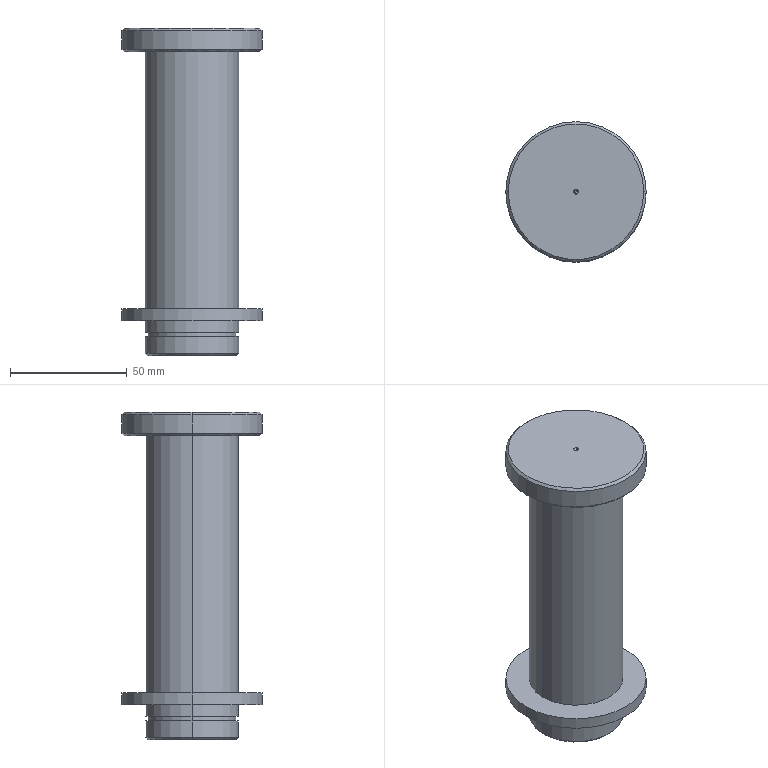Part | SolidWorks | features BaseBody 2 | 2 solids | 29 faces | box 60 x 60 x 140 mm | volume 198937 mm3 | cylinder 12 | cone 10 | plane 7 | commonest cylinder face diameters 40 x6 60 x4 37.5 x2
STEP:
#1=CARTESIAN_POINT('',(29.,0.,60.));
#2=VERTEX_POINT('',#1);
#3=CARTESIAN_POINT('',(-29.,0.,60.));
#4=VERTEX_POINT('',#3);
#5=CARTESIAN_POINT('',(0.,0.,60.));
#6=DIRECTION('',(0.,0.,1.));
#7=DIRECTION('',(1.,0.,0.));
#8=AXIS2_PLACEMENT_3D('',#5,#6,#7);
#9=CIRCLE('',#8,29.);
#10=EDGE_CURVE('',#2,#4,#9,.T.);
#11=ORIENTED_EDGE('',*,*,#10,.T.);
#12=CARTESIAN_POINT('',(-30.,0.,61.));
#13=VERTEX_POINT('',#12);
#14=CARTESIAN_POINT('',(-29.,0.,60.));
#15=DIRECTION('',(-0.7071,0.,0.7071));
#16=VECTOR('',#15,1000.);
#17=LINE('',#14,#16);
#18=EDGE_CURVE('',#4,#13,#17,.T.);
#19=ORIENTED_EDGE('',*,*,#18,.T.);
#20=CARTESIAN_POINT('',(30.,0.,61.));
#21=VERTEX_POINT('',#20);
#22=CARTESIAN_POINT('',(0.,0.,61.));
#23=DIRECTION('',(0.,0.,1.));
#24=DIRECTION('',(1.,0.,0.));
#25=AXIS2_PLACEMENT_3D('',#22,#23,#24);
#26=CIRCLE('',#25,30.);
#27=EDGE_CURVE('',#21,#13,#26,.T.);
#28=ORIENTED_EDGE('',*,*,#27,.F.);
#29=CARTESIAN_POINT('',(29.,0.,60.));
#30=DIRECTION('',(0.7071,0.,0.7071));
#31=VECTOR('',#30,1000.);
#32=LINE('',#29,#31);
#33=EDGE_CURVE('',#2,#21,#32,.T.);
#34=ORIENTED_EDGE('',*,*,#33,.F.);
#35=EDGE_LOOP('',(#11,#19,#28,#34));
#36=FACE_OUTER_BOUND('',#35,.T.);
#37=CARTESIAN_POINT('',(0.,0.,60.));
#38=DIRECTION('',(0.,0.,1.));
#39=DIRECTION('',(1.,0.,0.));
#40=AXIS2_PLACEMENT_3D('',#37,#38,#39);
#41=CONICAL_SURFACE('',#40,29.,0.7854);
#42=ADVANCED_FACE('',(#36),#41,.T.);
#43=ORIENTED_EDGE('',*,*,#27,.T.);
#44=CARTESIAN_POINT('',(-30.,0.,69.));
#45=VERTEX_POINT('',#44);
#46=CARTESIAN_POINT('',(-30.,0.,69.));
#47=DIRECTION('',(0.,0.,1.));
#48=VECTOR('',#47,1000.);
#49=LINE('',#46,#48);
#50=EDGE_CURVE('',#13,#45,#49,.T.);
#51=ORIENTED_EDGE('',*,*,#50,.T.);
#52=CARTESIAN_POINT('',(30.,0.,69.));
#53=VERTEX_POINT('',#52);
#54=CARTESIAN_POINT('',(0.,0.,69.));
#55=DIRECTION('',(0.,0.,1.));
#56=DIRECTION('',(1.,0.,0.));
#57=AXIS2_PLACEMENT_3D('',#54,#55,#56);
#58=CIRCLE('',#57,30.);
#59=EDGE_CURVE('',#53,#45,#58,.T.);
#60=ORIENTED_EDGE('',*,*,#59,.F.);
#61=CARTESIAN_POINT('',(30.,0.,69.));
#62=DIRECTION('',(0.,0.,1.));
#63=VECTOR('',#62,1000.);
#64=LINE('',#61,#63);
#65=EDGE_CURVE('',#21,#53,#64,.T.);
#66=ORIENTED_EDGE('',*,*,#65,.F.);
#67=EDGE_LOOP('',(#43,#51,#60,#66));
#68=FACE_OUTER_BOUND('',#67,.T.);
#69=CARTESIAN_POINT('',(0.,0.,69.));
#70=DIRECTION('',(0.,0.,1.));
#71=DIRECTION('',(1.,0.,0.));
#72=AXIS2_PLACEMENT_3D('',#69,#70,#71);
#73=CYLINDRICAL_SURFACE('',#72,30.);
#74=ADVANCED_FACE('',(#68),#73,.T.);
#75=CARTESIAN_POINT('',(29.,0.,70.));
#76=VERTEX_POINT('',#75);
#77=CARTESIAN_POINT('',(-29.,0.,70.));
#78=VERTEX_POINT('',#77);
#79=CARTESIAN_POINT('',(0.,0.,70.));
#80=DIRECTION('',(0.,0.,1.));
#81=DIRECTION('',(1.,0.,0.));
#82=AXIS2_PLACEMENT_3D('',#79,#80,#81);
#83=CIRCLE('',#82,29.);
#84=EDGE_CURVE('',#76,#78,#83,.T.);
#85=ORIENTED_EDGE('',*,*,#84,.F.);
#86=CARTESIAN_POINT('',(30.,0.,69.));
#87=DIRECTION('',(0.7071,0.,-0.7071));
#88=VECTOR('',#87,1000.);
#89=LINE('',#86,#88);
#90=EDGE_CURVE('',#76,#53,#89,.T.);
#91=ORIENTED_EDGE('',*,*,#90,.T.);
#92=ORIENTED_EDGE('',*,*,#59,.T.);
#93=CARTESIAN_POINT('',(-30.,0.,69.));
#94=DIRECTION('',(-0.7071,0.,-0.7071));
#95=VECTOR('',#94,1000.);
#96=LINE('',#93,#95);
#97=EDGE_CURVE('',#78,#45,#96,.T.);
#98=ORIENTED_EDGE('',*,*,#97,.F.);
#99=EDGE_LOOP('',(#85,#91,#92,#98));
#100=FACE_OUTER_BOUND('',#99,.T.);
#101=CARTESIAN_POINT('',(0.,0.,69.));
#102=DIRECTION('',(0.,0.,-1.));
#103=DIRECTION('',(-1.,0.,0.));
#104=AXIS2_PLACEMENT_3D('',#101,#102,#103);
#105=CONICAL_SURFACE('',#104,30.,0.7854);
#106=ADVANCED_FACE('',(#100),#105,.T.);
#107=CARTESIAN_POINT('',(0.,0.,69.));
#108=VERTEX_POINT('',#107);
#109=CARTESIAN_POINT('',(1.,0.,70.));
#110=VERTEX_POINT('',#109);
#111=CARTESIAN_POINT('',(1.,0.,70.));
#112=DIRECTION('',(0.7071,0.,0.7071));
#113=VECTOR('',#112,1000.);
#114=LINE('',#111,#113);
#115=EDGE_CURVE('',#108,#110,#114,.T.);
#116=ORIENTED_EDGE('',*,*,#115,.F.);
#117=CARTESIAN_POINT('',(-1.,0.,70.));
#118=VERTEX_POINT('',#117);
#119=CARTESIAN_POINT('',(-1.,0.,70.));
#120=DIRECTION('',(-0.7071,0.,0.7071));
#121=VECTOR('',#120,1000.);
#122=LINE('',#119,#121);
#123=EDGE_CURVE('',#108,#118,#122,.T.);
#124=ORIENTED_EDGE('',*,*,#123,.T.);
#125=CARTESIAN_POINT('',(0.,0.,70.));
#126=DIRECTION('',(0.,0.,1.));
#127=DIRECTION('',(1.,0.,0.));
#128=AXIS2_PLACEMENT_3D('',#125,#126,#127);
#129=CIRCLE('',#128,1.);
#130=EDGE_CURVE('',#118,#110,#129,.T.);
#131=ORIENTED_EDGE('',*,*,#130,.T.);
#132=EDGE_LOOP('',(#116,#124,#131));
#133=FACE_OUTER_BOUND('',#132,.T.);
#134=CARTESIAN_POINT('',(0.,0.,70.));
#135=DIRECTION('',(0.,0.,1.));
#136=DIRECTION('',(1.,0.,0.));
#137=AXIS2_PLACEMENT_3D('',#134,#135,#136);
#138=CONICAL_SURFACE('',#137,1.,0.7854);
#139=ADVANCED_FACE('',(#133),#138,.F.);
#140=CARTESIAN_POINT('',(0.,0.,-69.));
#141=VERTEX_POINT('',#140);
#142=CARTESIAN_POINT('',(-1.,0.,-70.));
#143=VERTEX_POINT('',#142);
#144=CARTESIAN_POINT('',(0.,0.,-69.));
#145=DIRECTION('',(-0.7071,0.,-0.7071));
#146=VECTOR('',#145,1000.);
#147=LINE('',#144,#146);
#148=EDGE_CURVE('',#141,#143,#147,.T.);
#149=ORIENTED_EDGE('',*,*,#148,.F.);
#150=CARTESIAN_POINT('',(1.,0.,-70.));
#151=VERTEX_POINT('',#150);
#152=CARTESIAN_POINT('',(0.,0.,-69.));
#153=DIRECTION('',(0.7071,0.,-0.7071));
#154=VECTOR('',#153,1000.);
#155=LINE('',#152,#154);
#156=EDGE_CURVE('',#141,#151,#155,.T.);
#157=ORIENTED_EDGE('',*,*,#156,.T.);
#158=CARTESIAN_POINT('',(0.,0.,-70.));
#159=DIRECTION('',(0.,0.,1.));
#160=DIRECTION('',(1.,0.,0.));
#161=AXIS2_PLACEMENT_3D('',#158,#159,#160);
#162=CIRCLE('',#161,1.);
#163=EDGE_CURVE('',#143,#151,#162,.T.);
#164=ORIENTED_EDGE('',*,*,#163,.F.);
#165=EDGE_LOOP('',(#149,#157,#164));
#166=FACE_OUTER_BOUND('',#165,.T.);
#167=CARTESIAN_POINT('',(0.,0.,-1069.));
#168=DIRECTION('',(0.,0.,-1.));
#169=DIRECTION('',(-1.,0.,0.));
#170=AXIS2_PLACEMENT_3D('',#167,#168,#169);
#171=CONICAL_SURFACE('',#170,1000.,0.7854);
#172=ADVANCED_FACE('',(#166),#171,.F.);
#173=CARTESIAN_POINT('',(19.,0.,-70.));
#174=VERTEX_POINT('',#173);
#175=CARTESIAN_POINT('',(-19.,0.,-70.));
#176=VERTEX_POINT('',#175);
#177=CARTESIAN_POINT('',(0.,0.,-70.));
#178=DIRECTION('',(0.,0.,1.));
#179=DIRECTION('',(1.,0.,0.));
#180=AXIS2_PLACEMENT_3D('',#177,#178,#179);
#181=CIRCLE('',#180,19.);
#182=EDGE_CURVE('',#174,#176,#181,.T.);
#183=ORIENTED_EDGE('',*,*,#182,.T.);
#184=CARTESIAN_POINT('',(-20.,0.,-69.));
#185=VERTEX_POINT('',#184);
#186=CARTESIAN_POINT('',(-19.,0.,-70.));
#187=DIRECTION('',(-0.7071,0.,0.7071));
#188=VECTOR('',#187,1000.);
#189=LINE('',#186,#188);
#190=EDGE_CURVE('',#176,#185,#189,.T.);
#191=ORIENTED_EDGE('',*,*,#190,.T.);
#192=CARTESIAN_POINT('',(20.,0.,-69.));
#193=VERTEX_POINT('',#192);
#194=CARTESIAN_POINT('',(0.,0.,-69.));
#195=DIRECTION('',(0.,0.,1.));
#196=DIRECTION('',(1.,0.,0.));
#197=AXIS2_PLACEMENT_3D('',#194,#195,#196);
#198=CIRCLE('',#197,20.);
#199=EDGE_CURVE('',#193,#185,#198,.T.);
#200=ORIENTED_EDGE('',*,*,#199,.F.);
#201=CARTESIAN_POINT('',(19.,0.,-70.));
#202=DIRECTION('',(0.7071,0.,0.7071));
#203=VECTOR('',#202,1000.);
#204=LINE('',#201,#203);
#205=EDGE_CURVE('',#174,#193,#204,.T.);
#206=ORIENTED_EDGE('',*,*,#205,.F.);
#207=EDGE_LOOP('',(#183,#191,#200,#206));
#208=FACE_OUTER_BOUND('',#207,.T.);
#209=CARTESIAN_POINT('',(0.,0.,-70.));
#210=DIRECTION('',(0.,0.,1.));
#211=DIRECTION('',(1.,0.,0.));
#212=AXIS2_PLACEMENT_3D('',#209,#210,#211);
#213=CONICAL_SURFACE('',#212,19.,0.7854);
#214=ADVANCED_FACE('',(#208),#213,.T.);
#215=ORIENTED_EDGE('',*,*,#199,.T.);
#216=CARTESIAN_POINT('',(-20.,0.,-62.));
#217=VERTEX_POINT('',#216);
#218=CARTESIAN_POINT('',(-20.,0.,69.));
#219=DIRECTION('',(0.,0.,1.));
#220=VECTOR('',#219,1000.);
#221=LINE('',#218,#220);
#222=EDGE_CURVE('',#185,#217,#221,.T.);
#223=ORIENTED_EDGE('',*,*,#222,.T.);
#224=CARTESIAN_POINT('',(20.,0.,-62.));
#225=VERTEX_POINT('',#224);
#226=CARTESIAN_POINT('',(0.,0.,-62.));
#227=DIRECTION('',(0.,0.,1.));
#228=DIRECTION('',(1.,0.,0.));
#229=AXIS2_PLACEMENT_3D('',#226,#227,#228);
#230=CIRCLE('',#229,20.);
#231=EDGE_CURVE('',#225,#217,#230,.T.);
#232=ORIENTED_EDGE('',*,*,#231,.F.);
#233=CARTESIAN_POINT('',(20.,0.,69.));
#234=DIRECTION('',(0.,0.,1.));
#235=VECTOR('',#234,1000.);
#236=LINE('',#233,#235);
#237=EDGE_CURVE('',#193,#225,#236,.T.);
#238=ORIENTED_EDGE('',*,*,#237,.F.);
#239=EDGE_LOOP('',(#215,#223,#232,#238));
#240=FACE_OUTER_BOUND('',#239,.T.);
#241=CARTESIAN_POINT('',(0.,0.,69.));
#242=DIRECTION('',(0.,0.,1.));
#243=DIRECTION('',(1.,0.,0.));
#244=AXIS2_PLACEMENT_3D('',#241,#242,#243);
#245=CYLINDRICAL_SURFACE('',#244,20.);
#246=ADVANCED_FACE('',(#240),#245,.T.);
#247=CARTESIAN_POINT('',(18.75,0.,-62.));
#248=VERTEX_POINT('',#247);
#249=CARTESIAN_POINT('',(-18.75,0.,-62.));
#250=VERTEX_POINT('',#249);
#251=CARTESIAN_POINT('',(0.,0.,-62.));
#252=DIRECTION('',(0.,0.,1.));
#253=DIRECTION('',(1.,0.,0.));
#254=AXIS2_PLACEMENT_3D('',#251,#252,#253);
#255=CIRCLE('',#254,18.75);
#256=EDGE_CURVE('',#248,#250,#255,.T.);
#257=ORIENTED_EDGE('',*,*,#256,.T.);
#258=CARTESIAN_POINT('',(-18.75,0.,-60.));
#259=VERTEX_POINT('',#258);
#260=CARTESIAN_POINT('',(-18.75,0.,69.));
#261=DIRECTION('',(0.,0.,1.));
#262=VECTOR('',#261,1000.);
#263=LINE('',#260,#262);
#264=EDGE_CURVE('',#250,#259,#263,.T.);
#265=ORIENTED_EDGE('',*,*,#264,.T.);
#266=CARTESIAN_POINT('',(18.75,0.,-60.));
#267=VERTEX_POINT('',#266);
#268=CARTESIAN_POINT('',(0.,0.,-60.));
#269=DIRECTION('',(0.,0.,1.));
#270=DIRECTION('',(1.,0.,0.));
#271=AXIS2_PLACEMENT_3D('',#268,#269,#270);
#272=CIRCLE('',#271,18.75);
#273=EDGE_CURVE('',#267,#259,#272,.T.);
#274=ORIENTED_EDGE('',*,*,#273,.F.);
#275=CARTESIAN_POINT('',(18.75,0.,69.));
#276=DIRECTION('',(0.,0.,1.));
#277=VECTOR('',#276,1000.);
#278=LINE('',#275,#277);
#279=EDGE_CURVE('',#248,#267,#278,.T.);
#280=ORIENTED_EDGE('',*,*,#279,.F.);
#281=EDGE_LOOP('',(#257,#265,#274,#280));
#282=FACE_OUTER_BOUND('',#281,.T.);
#283=CARTESIAN_POINT('',(0.,0.,69.));
#284=DIRECTION('',(0.,0.,1.));
#285=DIRECTION('',(1.,0.,0.));
#286=AXIS2_PLACEMENT_3D('',#283,#284,#285);
#287=CYLINDRICAL_SURFACE('',#286,18.75);
#288=ADVANCED_FACE('',(#282),#287,.T.);
#289=CARTESIAN_POINT('',(20.,0.,-60.));
#290=VERTEX_POINT('',#289);
#291=CARTESIAN_POINT('',(-20.,0.,-60.));
#292=VERTEX_POINT('',#291);
#293=CARTESIAN_POINT('',(0.,0.,-60.));
#294=DIRECTION('',(0.,0.,1.));
#295=DIRECTION('',(1.,0.,0.));
#296=AXIS2_PLACEMENT_3D('',#293,#294,#295);
#297=CIRCLE('',#296,20.);
#298=EDGE_CURVE('',#290,#292,#297,.T.);
#299=ORIENTED_EDGE('',*,*,#298,.T.);
#300=CARTESIAN_POINT('',(-20.,0.,60.));
#301=VERTEX_POINT('',#300);
#302=CARTESIAN_POINT('',(-20.,0.,69.));
#303=DIRECTION('',(0.,0.,1.));
#304=VECTOR('',#303,1000.);
#305=LINE('',#302,#304);
#306=EDGE_CURVE('',#292,#301,#305,.T.);
#307=ORIENTED_EDGE('',*,*,#306,.T.);
#308=CARTESIAN_POINT('',(20.,0.,60.));
#309=VERTEX_POINT('',#308);
#310=CARTESIAN_POINT('',(0.,0.,60.));
#311=DIRECTION('',(0.,0.,1.));
#312=DIRECTION('',(1.,0.,0.));
#313=AXIS2_PLACEMENT_3D('',#310,#311,#312);
#314=CIRCLE('',#313,20.);
#315=EDGE_CURVE('',#309,#301,#314,.T.);
#316=ORIENTED_EDGE('',*,*,#315,.F.);
#317=CARTESIAN_POINT('',(20.,0.,69.));
#318=DIRECTION('',(0.,0.,1.));
#319=VECTOR('',#318,1000.);
#320=LINE('',#317,#319);
#321=EDGE_CURVE('',#290,#309,#320,.T.);
#322=ORIENTED_EDGE('',*,*,#321,.F.);
#323=EDGE_LOOP('',(#299,#307,#316,#322));
#324=FACE_OUTER_BOUND('',#323,.T.);
#325=CARTESIAN_POINT('',(0.,0.,69.));
#326=DIRECTION('',(0.,0.,1.));
#327=DIRECTION('',(1.,0.,0.));
#328=AXIS2_PLACEMENT_3D('',#325,#326,#327);
#329=CYLINDRICAL_SURFACE('',#328,20.);
#330=ADVANCED_FACE('',(#324),#329,.T.);
#331=ORIENTED_EDGE('',*,*,#306,.F.);
#332=CARTESIAN_POINT('',(0.,0.,-60.));
#333=DIRECTION('',(0.,0.,1.));
#334=DIRECTION('',(1.,0.,0.));
#335=AXIS2_PLACEMENT_3D('',#332,#333,#334);
#336=CIRCLE('',#335,20.);
#337=EDGE_CURVE('',#292,#290,#336,.T.);
#338=ORIENTED_EDGE('',*,*,#337,.T.);
#339=ORIENTED_EDGE('',*,*,#321,.T.);
#340=CARTESIAN_POINT('',(0.,0.,60.));
#341=DIRECTION('',(0.,0.,1.));
#342=DIRECTION('',(1.,0.,0.));
#343=AXIS2_PLACEMENT_3D('',#340,#341,#342);
#344=CIRCLE('',#343,20.);
#345=EDGE_CURVE('',#301,#309,#344,.T.);
#346=ORIENTED_EDGE('',*,*,#345,.F.);
#347=EDGE_LOOP('',(#331,#338,#339,#346));
#348=FACE_OUTER_BOUND('',#347,.T.);
#349=CARTESIAN_POINT('',(0.,0.,69.));
#350=DIRECTION('',(0.,0.,1.));
#351=DIRECTION('',(1.,0.,0.));
#352=AXIS2_PLACEMENT_3D('',#349,#350,#351);
#353=CYLINDRICAL_SURFACE('',#352,20.);
#354=ADVANCED_FACE('',(#348),#353,.T.);
#355=ORIENTED_EDGE('',*,*,#298,.F.);
#356=ORIENTED_EDGE('',*,*,#337,.F.);
#357=EDGE_LOOP('',(#355,#356));
#358=FACE_OUTER_BOUND('',#357,.T.);
#359=ORIENTED_EDGE('',*,*,#273,.T.);
#360=CARTESIAN_POINT('',(0.,0.,-60.));
#361=DIRECTION('',(0.,0.,1.));
#362=DIRECTION('',(1.,0.,0.));
#363=AXIS2_PLACEMENT_3D('',#360,#361,#362);
#364=CIRCLE('',#363,18.75);
#365=EDGE_CURVE('',#259,#267,#364,.T.);
#366=ORIENTED_EDGE('',*,*,#365,.T.);
#367=EDGE_LOOP('',(#359,#366));
#368=FACE_BOUND('',#367,.T.);
#369=CARTESIAN_POINT('',(0.,20.,-60.));
#370=DIRECTION('',(0.,0.,1.));
#371=DIRECTION('',(1.,0.,0.));
#372=AXIS2_PLACEMENT_3D('',#369,#370,#371);
#373=PLANE('',#372);
#374=ADVANCED_FACE('',(#358,#368),#373,.F.);
#375=ORIENTED_EDGE('',*,*,#264,.F.);
#376=CARTESIAN_POINT('',(0.,0.,-62.));
#377=DIRECTION('',(0.,0.,1.));
#378=DIRECTION('',(1.,0.,0.));
#379=AXIS2_PLACEMENT_3D('',#376,#377,#378);
#380=CIRCLE('',#379,18.75);
#381=EDGE_CURVE('',#250,#248,#380,.T.);
#382=ORIENTED_EDGE('',*,*,#381,.T.);
#383=ORIENTED_EDGE('',*,*,#279,.T.);
#384=ORIENTED_EDGE('',*,*,#365,.F.);
#385=EDGE_LOOP('',(#375,#382,#383,#384));
#386=FACE_OUTER_BOUND('',#385,.T.);
#387=CARTESIAN_POINT('',(0.,0.,69.));
#388=DIRECTION('',(0.,0.,1.));
#389=DIRECTION('',(1.,0.,0.));
#390=AXIS2_PLACEMENT_3D('',#387,#388,#389);
#391=CYLINDRICAL_SURFACE('',#390,18.75);
#392=ADVANCED_FACE('',(#386),#391,.T.);
#393=ORIENTED_EDGE('',*,*,#256,.F.);
#394=ORIENTED_EDGE('',*,*,#381,.F.);
#395=EDGE_LOOP('',(#393,#394));
#396=FACE_BOUND('',#395,.T.);
#397=ORIENTED_EDGE('',*,*,#231,.T.);
#398=CARTESIAN_POINT('',(0.,0.,-62.));
#399=DIRECTION('',(0.,0.,1.));
#400=DIRECTION('',(1.,0.,0.));
#401=AXIS2_PLACEMENT_3D('',#398,#399,#400);
#402=CIRCLE('',#401,20.);
#403=EDGE_CURVE('',#217,#225,#402,.T.);
#404=ORIENTED_EDGE('',*,*,#403,.T.);
#405=EDGE_LOOP('',(#397,#404));
#406=FACE_OUTER_BOUND('',#405,.T.);
#407=CARTESIAN_POINT('',(0.,18.75,-62.));
#408=DIRECTION('',(0.,0.,-1.));
#409=DIRECTION('',(-1.,0.,0.));
#410=AXIS2_PLACEMENT_3D('',#407,#408,#409);
#411=PLANE('',#410);
#412=ADVANCED_FACE('',(#396,#406),#411,.F.);
#413=ORIENTED_EDGE('',*,*,#222,.F.);
#414=CARTESIAN_POINT('',(0.,0.,-69.));
#415=DIRECTION('',(0.,0.,1.));
#416=DIRECTION('',(1.,0.,0.));
#417=AXIS2_PLACEMENT_3D('',#414,#415,#416);
#418=CIRCLE('',#417,20.);
#419=EDGE_CURVE('',#185,#193,#418,.T.);
#420=ORIENTED_EDGE('',*,*,#419,.T.);
#421=ORIENTED_EDGE('',*,*,#237,.T.);
#422=ORIENTED_EDGE('',*,*,#403,.F.);
#423=EDGE_LOOP('',(#413,#420,#421,#422));
#424=FACE_OUTER_BOUND('',#423,.T.);
#425=CARTESIAN_POINT('',(0.,0.,69.));
#426=DIRECTION('',(0.,0.,1.));
#427=DIRECTION('',(1.,0.,0.));
#428=AXIS2_PLACEMENT_3D('',#425,#426,#427);
#429=CYLINDRICAL_SURFACE('',#428,20.);
#430=ADVANCED_FACE('',(#424),#429,.T.);
#431=ORIENTED_EDGE('',*,*,#190,.F.);
#432=CARTESIAN_POINT('',(0.,0.,-70.));
#433=DIRECTION('',(0.,0.,1.));
#434=DIRECTION('',(1.,0.,0.));
#435=AXIS2_PLACEMENT_3D('',#432,#433,#434);
#436=CIRCLE('',#435,19.);
#437=EDGE_CURVE('',#176,#174,#436,.T.);
#438=ORIENTED_EDGE('',*,*,#437,.T.);
#439=ORIENTED_EDGE('',*,*,#205,.T.);
#440=ORIENTED_EDGE('',*,*,#419,.F.);
#441=EDGE_LOOP('',(#431,#438,#439,#440));
#442=FACE_OUTER_BOUND('',#441,.T.);
#443=CARTESIAN_POINT('',(0.,0.,-70.));
#444=DIRECTION('',(0.,0.,1.));
#445=DIRECTION('',(1.,0.,0.));
#446=AXIS2_PLACEMENT_3D('',#443,#444,#445);
#447=CONICAL_SURFACE('',#446,19.,0.7854);
#448=ADVANCED_FACE('',(#442),#447,.T.);
#449=ORIENTED_EDGE('',*,*,#182,.F.);
#450=ORIENTED_EDGE('',*,*,#437,.F.);
#451=EDGE_LOOP('',(#449,#450));
#452=FACE_OUTER_BOUND('',#451,.T.);
#453=ORIENTED_EDGE('',*,*,#163,.T.);
#454=CARTESIAN_POINT('',(0.,0.,-70.));
#455=DIRECTION('',(0.,0.,1.));
#456=DIRECTION('',(1.,0.,0.));
#457=AXIS2_PLACEMENT_3D('',#454,#455,#456);
#458=CIRCLE('',#457,1.);
#459=EDGE_CURVE('',#151,#143,#458,.T.);
#460=ORIENTED_EDGE('',*,*,#459,.T.);
#461=EDGE_LOOP('',(#453,#460));
#462=FACE_BOUND('',#461,.T.);
#463=CARTESIAN_POINT('',(0.,19.,-70.));
#464=DIRECTION('',(0.,0.,1.));
#465=DIRECTION('',(1.,0.,0.));
#466=AXIS2_PLACEMENT_3D('',#463,#464,#465);
#467=PLANE('',#466);
#468=ADVANCED_FACE('',(#452,#462),#467,.F.);
#469=ORIENTED_EDGE('',*,*,#156,.F.);
#470=ORIENTED_EDGE('',*,*,#148,.T.);
#471=ORIENTED_EDGE('',*,*,#459,.F.);
#472=EDGE_LOOP('',(#469,#470,#471));
#473=FACE_OUTER_BOUND('',#472,.T.);
#474=CARTESIAN_POINT('',(0.,0.,-1069.));
#475=DIRECTION('',(0.,0.,-1.));
#476=DIRECTION('',(-1.,0.,0.));
#477=AXIS2_PLACEMENT_3D('',#474,#475,#476);
#478=CONICAL_SURFACE('',#477,1000.,0.7854);
#479=ADVANCED_FACE('',(#473),#478,.F.);
#480=ORIENTED_EDGE('',*,*,#123,.F.);
#481=ORIENTED_EDGE('',*,*,#115,.T.);
#482=CARTESIAN_POINT('',(0.,0.,70.));
#483=DIRECTION('',(0.,0.,1.));
#484=DIRECTION('',(1.,0.,0.));
#485=AXIS2_PLACEMENT_3D('',#482,#483,#484);
#486=CIRCLE('',#485,1.);
#487=EDGE_CURVE('',#110,#118,#486,.T.);
#488=ORIENTED_EDGE('',*,*,#487,.T.);
#489=EDGE_LOOP('',(#480,#481,#488));
#490=FACE_OUTER_BOUND('',#489,.T.);
#491=CARTESIAN_POINT('',(0.,0.,70.));
#492=DIRECTION('',(0.,0.,1.));
#493=DIRECTION('',(1.,0.,0.));
#494=AXIS2_PLACEMENT_3D('',#491,#492,#493);
#495=CONICAL_SURFACE('',#494,1.,0.7854);
#496=ADVANCED_FACE('',(#490),#495,.F.);
#497=ORIENTED_EDGE('',*,*,#487,.F.);
#498=ORIENTED_EDGE('',*,*,#130,.F.);
#499=EDGE_LOOP('',(#497,#498));
#500=FACE_BOUND('',#499,.T.);
#501=CARTESIAN_POINT('',(0.,0.,70.));
#502=DIRECTION('',(0.,0.,1.));
#503=DIRECTION('',(1.,0.,0.));
#504=AXIS2_PLACEMENT_3D('',#501,#502,#503);
#505=CIRCLE('',#504,29.);
#506=EDGE_CURVE('',#78,#76,#505,.T.);
#507=ORIENTED_EDGE('',*,*,#506,.T.);
#508=ORIENTED_EDGE('',*,*,#84,.T.);
#509=EDGE_LOOP('',(#507,#508));
#510=FACE_OUTER_BOUND('',#509,.T.);
#511=CARTESIAN_POINT('',(0.,1.,70.));
#512=DIRECTION('',(0.,0.,-1.));
#513=DIRECTION('',(-1.,0.,0.));
#514=AXIS2_PLACEMENT_3D('',#511,#512,#513);
#515=PLANE('',#514);
#516=ADVANCED_FACE('',(#500,#510),#515,.F.);
#517=ORIENTED_EDGE('',*,*,#90,.F.);
#518=ORIENTED_EDGE('',*,*,#506,.F.);
#519=ORIENTED_EDGE('',*,*,#97,.T.);
#520=CARTESIAN_POINT('',(0.,0.,69.));
#521=DIRECTION('',(0.,0.,1.));
#522=DIRECTION('',(1.,0.,0.));
#523=AXIS2_PLACEMENT_3D('',#520,#521,#522);
#524=CIRCLE('',#523,30.);
#525=EDGE_CURVE('',#45,#53,#524,.T.);
#526=ORIENTED_EDGE('',*,*,#525,.T.);
#527=EDGE_LOOP('',(#517,#518,#519,#526));
#528=FACE_OUTER_BOUND('',#527,.T.);
#529=CARTESIAN_POINT('',(0.,0.,69.));
#530=DIRECTION('',(0.,0.,-1.));
#531=DIRECTION('',(-1.,0.,0.));
#532=AXIS2_PLACEMENT_3D('',#529,#530,#531);
#533=CONICAL_SURFACE('',#532,30.,0.7854);
#534=ADVANCED_FACE('',(#528),#533,.T.);
#535=ORIENTED_EDGE('',*,*,#50,.F.);
#536=CARTESIAN_POINT('',(0.,0.,61.));
#537=DIRECTION('',(0.,0.,1.));
#538=DIRECTION('',(1.,0.,0.));
#539=AXIS2_PLACEMENT_3D('',#536,#537,#538);
#540=CIRCLE('',#539,30.);
#541=EDGE_CURVE('',#13,#21,#540,.T.);
#542=ORIENTED_EDGE('',*,*,#541,.T.);
#543=ORIENTED_EDGE('',*,*,#65,.T.);
#544=ORIENTED_EDGE('',*,*,#525,.F.);
#545=EDGE_LOOP('',(#535,#542,#543,#544));
#546=FACE_OUTER_BOUND('',#545,.T.);
#547=CARTESIAN_POINT('',(0.,0.,69.));
#548=DIRECTION('',(0.,0.,1.));
#549=DIRECTION('',(1.,0.,0.));
#550=AXIS2_PLACEMENT_3D('',#547,#548,#549);
#551=CYLINDRICAL_SURFACE('',#550,30.);
#552=ADVANCED_FACE('',(#546),#551,.T.);
#553=ORIENTED_EDGE('',*,*,#18,.F.);
#554=CARTESIAN_POINT('',(0.,0.,60.));
#555=DIRECTION('',(0.,0.,1.));
#556=DIRECTION('',(1.,0.,0.));
#557=AXIS2_PLACEMENT_3D('',#554,#555,#556);
#558=CIRCLE('',#557,29.);
#559=EDGE_CURVE('',#4,#2,#558,.T.);
#560=ORIENTED_EDGE('',*,*,#559,.T.);
#561=ORIENTED_EDGE('',*,*,#33,.T.);
#562=ORIENTED_EDGE('',*,*,#541,.F.);
#563=EDGE_LOOP('',(#553,#560,#561,#562));
#564=FACE_OUTER_BOUND('',#563,.T.);
#565=CARTESIAN_POINT('',(0.,0.,60.));
#566=DIRECTION('',(0.,0.,1.));
#567=DIRECTION('',(1.,0.,0.));
#568=AXIS2_PLACEMENT_3D('',#565,#566,#567);
#569=CONICAL_SURFACE('',#568,29.,0.7854);
#570=ADVANCED_FACE('',(#564),#569,.T.);
#571=ORIENTED_EDGE('',*,*,#10,.F.);
#572=ORIENTED_EDGE('',*,*,#559,.F.);
#573=EDGE_LOOP('',(#571,#572));
#574=FACE_OUTER_BOUND('',#573,.T.);
#575=ORIENTED_EDGE('',*,*,#315,.T.);
#576=ORIENTED_EDGE('',*,*,#345,.T.);
#577=EDGE_LOOP('',(#575,#576));
#578=FACE_BOUND('',#577,.T.);
#579=CARTESIAN_POINT('',(0.,29.,60.));
#580=DIRECTION('',(0.,0.,1.));
#581=DIRECTION('',(1.,0.,0.));
#582=AXIS2_PLACEMENT_3D('',#579,#580,#581);
#583=PLANE('',#582);
#584=ADVANCED_FACE('',(#574,#578),#583,.F.);
#585=CLOSED_SHELL('',(#42,#74,#106,#139,#172,#214,#246,#288,#330,#354,#374,#392,#412,#430,#448,#468,#479,#496,#516,#534,#552,#570,#584));
#586=MANIFOLD_SOLID_BREP('',#585);
#587=CARTESIAN_POINT('',(20.,0.,-50.));
#588=VERTEX_POINT('',#587);
#589=CARTESIAN_POINT('',(-20.,0.,-50.));
#590=VERTEX_POINT('',#589);
#591=CARTESIAN_POINT('',(0.,0.,-50.));
#592=DIRECTION('',(0.,0.,-1.));
#593=DIRECTION('',(-1.,0.,0.));
#594=AXIS2_PLACEMENT_3D('',#591,#592,#593);
#595=CIRCLE('',#594,20.);
#596=EDGE_CURVE('',#588,#590,#595,.T.);
#597=ORIENTED_EDGE('',*,*,#596,.F.);
#598=CARTESIAN_POINT('',(20.,0.,-55.));
#599=VERTEX_POINT('',#598);
#600=CARTESIAN_POINT('',(20.,0.,-50.));
#601=DIRECTION('',(0.,0.,-1.));
#602=VECTOR('',#601,1000.);
#603=LINE('',#600,#602);
#604=EDGE_CURVE('',#588,#599,#603,.T.);
#605=ORIENTED_EDGE('',*,*,#604,.T.);
#606=CARTESIAN_POINT('',(-20.,0.,-55.));
#607=VERTEX_POINT('',#606);
#608=CARTESIAN_POINT('',(0.,0.,-55.));
#609=DIRECTION('',(0.,0.,-1.));
#610=DIRECTION('',(-1.,0.,0.));
#611=AXIS2_PLACEMENT_3D('',#608,#609,#610);
#612=CIRCLE('',#611,20.);
#613=EDGE_CURVE('',#599,#607,#612,.T.);
#614=ORIENTED_EDGE('',*,*,#613,.T.);
#615=CARTESIAN_POINT('',(-20.,0.,-50.));
#616=DIRECTION('',(0.,0.,-1.));
#617=VECTOR('',#616,1000.);
#618=LINE('',#615,#617);
#619=EDGE_CURVE('',#590,#607,#618,.T.);
#620=ORIENTED_EDGE('',*,*,#619,.F.);
#621=EDGE_LOOP('',(#597,#605,#614,#620));
#622=FACE_OUTER_BOUND('',#621,.T.);
#623=CARTESIAN_POINT('',(0.,0.,-50.));
#624=DIRECTION('',(0.,0.,-1.));
#625=DIRECTION('',(-1.,0.,0.));
#626=AXIS2_PLACEMENT_3D('',#623,#624,#625);
#627=CYLINDRICAL_SURFACE('',#626,20.);
#628=ADVANCED_FACE('',(#622),#627,.F.);
#629=CARTESIAN_POINT('',(-30.,0.,-50.));
#630=VERTEX_POINT('',#629);
#631=CARTESIAN_POINT('',(30.,0.,-50.));
#632=VERTEX_POINT('',#631);
#633=CARTESIAN_POINT('',(0.,0.,-50.));
#634=DIRECTION('',(0.,0.,-1.));
#635=DIRECTION('',(-1.,0.,0.));
#636=AXIS2_PLACEMENT_3D('',#633,#634,#635);
#637=CIRCLE('',#636,30.);
#638=EDGE_CURVE('',#630,#632,#637,.T.);
#639=ORIENTED_EDGE('',*,*,#638,.T.);
#640=CARTESIAN_POINT('',(30.,0.,-55.));
#641=VERTEX_POINT('',#640);
#642=CARTESIAN_POINT('',(30.,0.,-50.));
#643=DIRECTION('',(0.,0.,-1.));
#644=VECTOR('',#643,1000.);
#645=LINE('',#642,#644);
#646=EDGE_CURVE('',#632,#641,#645,.T.);
#647=ORIENTED_EDGE('',*,*,#646,.T.);
#648=CARTESIAN_POINT('',(-30.,0.,-55.));
#649=VERTEX_POINT('',#648);
#650=CARTESIAN_POINT('',(0.,0.,-55.));
#651=DIRECTION('',(0.,0.,-1.));
#652=DIRECTION('',(-1.,0.,0.));
#653=AXIS2_PLACEMENT_3D('',#650,#651,#652);
#654=CIRCLE('',#653,30.);
#655=EDGE_CURVE('',#649,#641,#654,.T.);
#656=ORIENTED_EDGE('',*,*,#655,.F.);
#657=CARTESIAN_POINT('',(-30.,0.,-50.));
#658=DIRECTION('',(0.,0.,-1.));
#659=VECTOR('',#658,1000.);
#660=LINE('',#657,#659);
#661=EDGE_CURVE('',#630,#649,#660,.T.);
#662=ORIENTED_EDGE('',*,*,#661,.F.);
#663=EDGE_LOOP('',(#639,#647,#656,#662));
#664=FACE_OUTER_BOUND('',#663,.T.);
#665=CARTESIAN_POINT('',(0.,0.,-50.));
#666=DIRECTION('',(0.,0.,-1.));
#667=DIRECTION('',(-1.,0.,0.));
#668=AXIS2_PLACEMENT_3D('',#665,#666,#667);
#669=CYLINDRICAL_SURFACE('',#668,30.);
#670=ADVANCED_FACE('',(#664),#669,.T.);
#671=ORIENTED_EDGE('',*,*,#646,.F.);
#672=CARTESIAN_POINT('',(0.,0.,-50.));
#673=DIRECTION('',(0.,0.,-1.));
#674=DIRECTION('',(-1.,0.,0.));
#675=AXIS2_PLACEMENT_3D('',#672,#673,#674);
#676=CIRCLE('',#675,30.);
#677=EDGE_CURVE('',#632,#630,#676,.T.);
#678=ORIENTED_EDGE('',*,*,#677,.T.);
#679=ORIENTED_EDGE('',*,*,#661,.T.);
#680=CARTESIAN_POINT('',(0.,0.,-55.));
#681=DIRECTION('',(0.,0.,-1.));
#682=DIRECTION('',(-1.,0.,0.));
#683=AXIS2_PLACEMENT_3D('',#680,#681,#682);
#684=CIRCLE('',#683,30.);
#685=EDGE_CURVE('',#641,#649,#684,.T.);
#686=ORIENTED_EDGE('',*,*,#685,.F.);
#687=EDGE_LOOP('',(#671,#678,#679,#686));
#688=FACE_OUTER_BOUND('',#687,.T.);
#689=CARTESIAN_POINT('',(0.,0.,-50.));
#690=DIRECTION('',(0.,0.,-1.));
#691=DIRECTION('',(-1.,0.,0.));
#692=AXIS2_PLACEMENT_3D('',#689,#690,#691);
#693=CYLINDRICAL_SURFACE('',#692,30.);
#694=ADVANCED_FACE('',(#688),#693,.T.);
#695=CARTESIAN_POINT('',(0.,0.,-50.));
#696=DIRECTION('',(0.,0.,-1.));
#697=DIRECTION('',(-1.,0.,0.));
#698=AXIS2_PLACEMENT_3D('',#695,#696,#697);
#699=CIRCLE('',#698,20.);
#700=EDGE_CURVE('',#590,#588,#699,.T.);
#701=ORIENTED_EDGE('',*,*,#700,.T.);
#702=ORIENTED_EDGE('',*,*,#596,.T.);
#703=EDGE_LOOP('',(#701,#702));
#704=FACE_BOUND('',#703,.T.);
#705=ORIENTED_EDGE('',*,*,#638,.F.);
#706=ORIENTED_EDGE('',*,*,#677,.F.);
#707=EDGE_LOOP('',(#705,#706));
#708=FACE_OUTER_BOUND('',#707,.T.);
#709=CARTESIAN_POINT('',(0.,0.,-50.));
#710=DIRECTION('',(0.,0.,-1.));
#711=DIRECTION('',(-1.,0.,0.));
#712=AXIS2_PLACEMENT_3D('',#709,#710,#711);
#713=PLANE('',#712);
#714=ADVANCED_FACE('',(#704,#708),#713,.F.);
#715=CARTESIAN_POINT('',(0.,0.,-55.));
#716=DIRECTION('',(0.,0.,-1.));
#717=DIRECTION('',(-1.,0.,0.));
#718=AXIS2_PLACEMENT_3D('',#715,#716,#717);
#719=CIRCLE('',#718,20.);
#720=EDGE_CURVE('',#607,#599,#719,.T.);
#721=ORIENTED_EDGE('',*,*,#720,.F.);
#722=ORIENTED_EDGE('',*,*,#613,.F.);
#723=EDGE_LOOP('',(#721,#722));
#724=FACE_BOUND('',#723,.T.);
#725=ORIENTED_EDGE('',*,*,#655,.T.);
#726=ORIENTED_EDGE('',*,*,#685,.T.);
#727=EDGE_LOOP('',(#725,#726));
#728=FACE_OUTER_BOUND('',#727,.T.);
#729=CARTESIAN_POINT('',(0.,0.,-55.));
#730=DIRECTION('',(0.,0.,-1.));
#731=DIRECTION('',(-1.,0.,0.));
#732=AXIS2_PLACEMENT_3D('',#729,#730,#731);
#733=PLANE('',#732);
#734=ADVANCED_FACE('',(#724,#728),#733,.T.);
#735=ORIENTED_EDGE('',*,*,#604,.F.);
#736=ORIENTED_EDGE('',*,*,#700,.F.);
#737=ORIENTED_EDGE('',*,*,#619,.T.);
#738=ORIENTED_EDGE('',*,*,#720,.T.);
#739=EDGE_LOOP('',(#735,#736,#737,#738));
#740=FACE_OUTER_BOUND('',#739,.T.);
#741=CARTESIAN_POINT('',(0.,0.,-50.));
#742=DIRECTION('',(0.,0.,-1.));
#743=DIRECTION('',(-1.,0.,0.));
#744=AXIS2_PLACEMENT_3D('',#741,#742,#743);
#745=CYLINDRICAL_SURFACE('',#744,20.);
#746=ADVANCED_FACE('',(#740),#745,.F.);
#747=CLOSED_SHELL('',(#628,#670,#694,#714,#734,#746));
#748=MANIFOLD_SOLID_BREP('',#747);
#749=CARTESIAN_POINT('',(0.,0.,0.));
#750=DIRECTION('',(0.,0.,1.));
#751=DIRECTION('',(1.,0.,0.));
#752=AXIS2_PLACEMENT_3D('',#749,#750,#751);
#753=(LENGTH_UNIT()NAMED_UNIT(*)SI_UNIT(.MILLI.,.METRE.));
#754=UNCERTAINTY_MEASURE_WITH_UNIT(LENGTH_MEASURE(0.00001),#753,'','');
#755=(NAMED_UNIT(*)PLANE_ANGLE_UNIT()SI_UNIT($,.RADIAN.));
#756=(NAMED_UNIT(*)SI_UNIT($,.STERADIAN.)SOLID_ANGLE_UNIT());
#757=(GEOMETRIC_REPRESENTATION_CONTEXT(3)GLOBAL_UNCERTAINTY_ASSIGNED_CONTEXT((#754))GLOBAL_UNIT_ASSIGNED_CONTEXT((#753,#755,#756))REPRESENTATION_CONTEXT('',''));
#758=ADVANCED_BREP_SHAPE_REPRESENTATION('',(#586,#748,#752),#757);